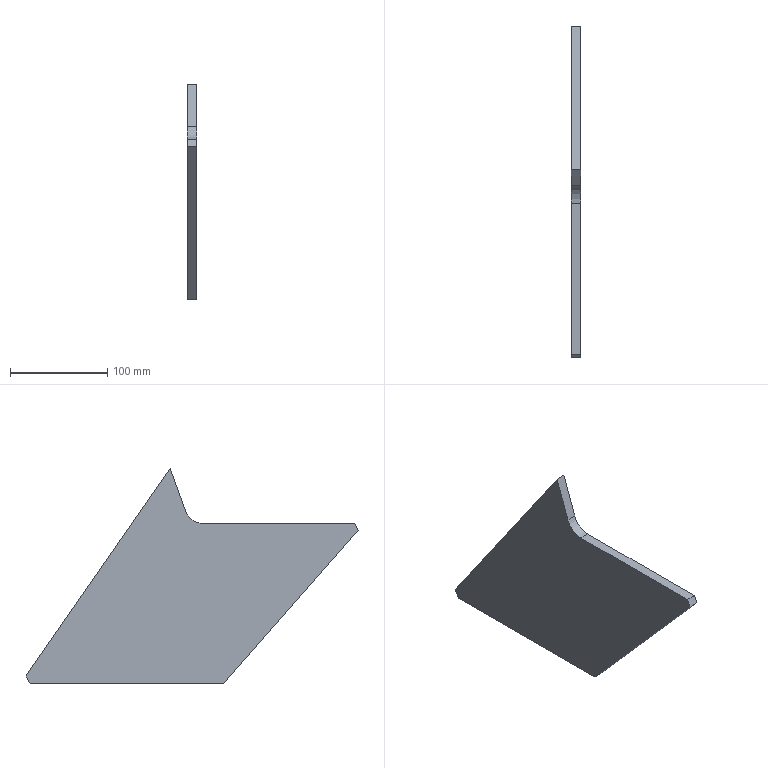Part | SolidWorks | features Extrusion 1 | 1 solid | 10 faces | box 10 x 341.699 x 222 mm | volume 386732 mm3 | plane 9 | cylinder 1 | commonest cylinder face diameters 40 x1
STEP:
#1=CARTESIAN_POINT('',(0.,6.601,157.488));
#2=VERTEX_POINT('',#1);
#3=CARTESIAN_POINT('',(0.,145.,0.));
#4=VERTEX_POINT('',#3);
#5=CARTESIAN_POINT('',(0.,6.601,157.488));
#6=DIRECTION('',(0.,0.6601,-0.7512));
#7=VECTOR('',#6,1000.);
#8=LINE('',#5,#7);
#9=EDGE_CURVE('',#2,#4,#8,.T.);
#10=ORIENTED_EDGE('',*,*,#9,.T.);
#11=CARTESIAN_POINT('',(10.,145.,0.));
#12=VERTEX_POINT('',#11);
#13=CARTESIAN_POINT('',(10.,145.,0.));
#14=DIRECTION('',(-1.,0.,0.));
#15=VECTOR('',#14,1000.);
#16=LINE('',#13,#15);
#17=EDGE_CURVE('',#12,#4,#16,.T.);
#18=ORIENTED_EDGE('',*,*,#17,.F.);
#19=CARTESIAN_POINT('',(10.,6.601,157.488));
#20=VERTEX_POINT('',#19);
#21=CARTESIAN_POINT('',(10.,6.601,157.488));
#22=DIRECTION('',(0.,0.6601,-0.7512));
#23=VECTOR('',#22,1000.);
#24=LINE('',#21,#23);
#25=EDGE_CURVE('',#20,#12,#24,.T.);
#26=ORIENTED_EDGE('',*,*,#25,.F.);
#27=CARTESIAN_POINT('',(10.,6.601,157.488));
#28=DIRECTION('',(-1.,0.,0.));
#29=VECTOR('',#28,1000.);
#30=LINE('',#27,#29);
#31=EDGE_CURVE('',#20,#2,#30,.T.);
#32=ORIENTED_EDGE('',*,*,#31,.T.);
#33=EDGE_LOOP('',(#10,#18,#26,#32));
#34=FACE_OUTER_BOUND('',#33,.T.);
#35=CARTESIAN_POINT('',(10.,6.601,157.488));
#36=DIRECTION('',(0.,0.7512,0.6601));
#37=DIRECTION('',(0.,-0.6601,0.7512));
#38=AXIS2_PLACEMENT_3D('',#35,#36,#37);
#39=PLANE('',#38);
#40=ADVANCED_FACE('',(#34),#39,.F.);
#41=CARTESIAN_POINT('',(0.,344.,0.));
#42=VERTEX_POINT('',#41);
#43=CARTESIAN_POINT('',(0.,145.,0.));
#44=DIRECTION('',(0.,1.,0.));
#45=VECTOR('',#44,1000.);
#46=LINE('',#43,#45);
#47=EDGE_CURVE('',#4,#42,#46,.T.);
#48=ORIENTED_EDGE('',*,*,#47,.T.);
#49=CARTESIAN_POINT('',(10.,344.,0.));
#50=VERTEX_POINT('',#49);
#51=CARTESIAN_POINT('',(10.,344.,0.));
#52=DIRECTION('',(-1.,0.,0.));
#53=VECTOR('',#52,1000.);
#54=LINE('',#51,#53);
#55=EDGE_CURVE('',#50,#42,#54,.T.);
#56=ORIENTED_EDGE('',*,*,#55,.F.);
#57=CARTESIAN_POINT('',(10.,145.,0.));
#58=DIRECTION('',(0.,1.,0.));
#59=VECTOR('',#58,1000.);
#60=LINE('',#57,#59);
#61=EDGE_CURVE('',#12,#50,#60,.T.);
#62=ORIENTED_EDGE('',*,*,#61,.F.);
#63=ORIENTED_EDGE('',*,*,#17,.T.);
#64=EDGE_LOOP('',(#48,#56,#62,#63));
#65=FACE_OUTER_BOUND('',#64,.T.);
#66=CARTESIAN_POINT('',(10.,145.,0.));
#67=DIRECTION('',(0.,0.,1.));
#68=DIRECTION('',(1.,0.,0.));
#69=AXIS2_PLACEMENT_3D('',#66,#67,#68);
#70=PLANE('',#69);
#71=ADVANCED_FACE('',(#65),#70,.F.);
#72=CARTESIAN_POINT('',(0.,348.3,8.217));
#73=VERTEX_POINT('',#72);
#74=CARTESIAN_POINT('',(0.,344.,0.));
#75=DIRECTION('',(0.,0.4637,0.886));
#76=VECTOR('',#75,1000.);
#77=LINE('',#74,#76);
#78=EDGE_CURVE('',#42,#73,#77,.T.);
#79=ORIENTED_EDGE('',*,*,#78,.T.);
#80=CARTESIAN_POINT('',(10.,348.3,8.217));
#81=VERTEX_POINT('',#80);
#82=CARTESIAN_POINT('',(10.,348.3,8.217));
#83=DIRECTION('',(-1.,0.,0.));
#84=VECTOR('',#83,1000.);
#85=LINE('',#82,#84);
#86=EDGE_CURVE('',#81,#73,#85,.T.);
#87=ORIENTED_EDGE('',*,*,#86,.F.);
#88=CARTESIAN_POINT('',(10.,344.,0.));
#89=DIRECTION('',(0.,0.4637,0.886));
#90=VECTOR('',#89,1000.);
#91=LINE('',#88,#90);
#92=EDGE_CURVE('',#50,#81,#91,.T.);
#93=ORIENTED_EDGE('',*,*,#92,.F.);
#94=ORIENTED_EDGE('',*,*,#55,.T.);
#95=EDGE_LOOP('',(#79,#87,#93,#94));
#96=FACE_OUTER_BOUND('',#95,.T.);
#97=CARTESIAN_POINT('',(10.,344.,0.));
#98=DIRECTION('',(0.,-0.886,0.4637));
#99=DIRECTION('',(0.,-0.4637,-0.886));
#100=AXIS2_PLACEMENT_3D('',#97,#98,#99);
#101=PLANE('',#100);
#102=ADVANCED_FACE('',(#96),#101,.F.);
#103=CARTESIAN_POINT('',(0.,200.,222.));
#104=VERTEX_POINT('',#103);
#105=CARTESIAN_POINT('',(0.,348.3,8.217));
#106=DIRECTION('',(0.,-0.57,0.8217));
#107=VECTOR('',#106,1000.);
#108=LINE('',#105,#107);
#109=EDGE_CURVE('',#73,#104,#108,.T.);
#110=ORIENTED_EDGE('',*,*,#109,.T.);
#111=CARTESIAN_POINT('',(10.,200.,222.));
#112=VERTEX_POINT('',#111);
#113=CARTESIAN_POINT('',(10.,200.,222.));
#114=DIRECTION('',(-1.,0.,0.));
#115=VECTOR('',#114,1000.);
#116=LINE('',#113,#115);
#117=EDGE_CURVE('',#112,#104,#116,.T.);
#118=ORIENTED_EDGE('',*,*,#117,.F.);
#119=CARTESIAN_POINT('',(10.,348.3,8.217));
#120=DIRECTION('',(0.,-0.57,0.8217));
#121=VECTOR('',#120,1000.);
#122=LINE('',#119,#121);
#123=EDGE_CURVE('',#81,#112,#122,.T.);
#124=ORIENTED_EDGE('',*,*,#123,.F.);
#125=ORIENTED_EDGE('',*,*,#86,.T.);
#126=EDGE_LOOP('',(#110,#118,#124,#125));
#127=FACE_OUTER_BOUND('',#126,.T.);
#128=CARTESIAN_POINT('',(10.,348.3,8.217));
#129=DIRECTION('',(0.,-0.8217,-0.57));
#130=DIRECTION('',(0.,0.57,-0.8217));
#131=AXIS2_PLACEMENT_3D('',#128,#129,#130);
#132=PLANE('',#131);
#133=ADVANCED_FACE('',(#127),#132,.F.);
#134=CARTESIAN_POINT('',(0.,184.259,178.231));
#135=VERTEX_POINT('',#134);
#136=CARTESIAN_POINT('',(0.,200.,222.));
#137=DIRECTION('',(0.,-0.3384,-0.941));
#138=VECTOR('',#137,1000.);
#139=LINE('',#136,#138);
#140=EDGE_CURVE('',#104,#135,#139,.T.);
#141=ORIENTED_EDGE('',*,*,#140,.T.);
#142=CARTESIAN_POINT('',(10.,184.259,178.231));
#143=VERTEX_POINT('',#142);
#144=CARTESIAN_POINT('',(10.,184.259,178.231));
#145=DIRECTION('',(-1.,0.,0.));
#146=VECTOR('',#145,1000.);
#147=LINE('',#144,#146);
#148=EDGE_CURVE('',#143,#135,#147,.T.);
#149=ORIENTED_EDGE('',*,*,#148,.F.);
#150=CARTESIAN_POINT('',(10.,200.,222.));
#151=DIRECTION('',(0.,-0.3384,-0.941));
#152=VECTOR('',#151,1000.);
#153=LINE('',#150,#152);
#154=EDGE_CURVE('',#112,#143,#153,.T.);
#155=ORIENTED_EDGE('',*,*,#154,.F.);
#156=ORIENTED_EDGE('',*,*,#117,.T.);
#157=EDGE_LOOP('',(#141,#149,#155,#156));
#158=FACE_OUTER_BOUND('',#157,.T.);
#159=CARTESIAN_POINT('',(10.,200.,222.));
#160=DIRECTION('',(0.,0.941,-0.3384));
#161=DIRECTION('',(0.,0.3384,0.941));
#162=AXIS2_PLACEMENT_3D('',#159,#160,#161);
#163=PLANE('',#162);
#164=ADVANCED_FACE('',(#158),#163,.F.);
#165=CARTESIAN_POINT('',(0.,165.439,165.));
#166=VERTEX_POINT('',#165);
#167=CARTESIAN_POINT('',(0.,165.439,185.));
#168=DIRECTION('',(-1.,0.,0.));
#169=DIRECTION('',(0.,0.,1.));
#170=AXIS2_PLACEMENT_3D('',#167,#168,#169);
#171=CIRCLE('',#170,20.);
#172=EDGE_CURVE('',#135,#166,#171,.T.);
#173=ORIENTED_EDGE('',*,*,#172,.T.);
#174=CARTESIAN_POINT('',(10.,165.439,165.));
#175=VERTEX_POINT('',#174);
#176=CARTESIAN_POINT('',(10.,165.439,165.));
#177=DIRECTION('',(-1.,0.,0.));
#178=VECTOR('',#177,1000.);
#179=LINE('',#176,#178);
#180=EDGE_CURVE('',#175,#166,#179,.T.);
#181=ORIENTED_EDGE('',*,*,#180,.F.);
#182=CARTESIAN_POINT('',(10.,165.439,185.));
#183=DIRECTION('',(-1.,0.,0.));
#184=DIRECTION('',(0.,0.,1.));
#185=AXIS2_PLACEMENT_3D('',#182,#183,#184);
#186=CIRCLE('',#185,20.);
#187=EDGE_CURVE('',#143,#175,#186,.T.);
#188=ORIENTED_EDGE('',*,*,#187,.F.);
#189=ORIENTED_EDGE('',*,*,#148,.T.);
#190=EDGE_LOOP('',(#173,#181,#188,#189));
#191=FACE_OUTER_BOUND('',#190,.T.);
#192=CARTESIAN_POINT('',(10.,165.439,185.));
#193=DIRECTION('',(-1.,0.,0.));
#194=DIRECTION('',(0.,0.,1.));
#195=AXIS2_PLACEMENT_3D('',#192,#193,#194);
#196=CYLINDRICAL_SURFACE('',#195,20.);
#197=ADVANCED_FACE('',(#191),#196,.F.);
#198=CARTESIAN_POINT('',(0.,10.,165.));
#199=VERTEX_POINT('',#198);
#200=CARTESIAN_POINT('',(0.,165.439,165.));
#201=DIRECTION('',(0.,-1.,0.));
#202=VECTOR('',#201,1000.);
#203=LINE('',#200,#202);
#204=EDGE_CURVE('',#166,#199,#203,.T.);
#205=ORIENTED_EDGE('',*,*,#204,.T.);
#206=CARTESIAN_POINT('',(10.,10.,165.));
#207=VERTEX_POINT('',#206);
#208=CARTESIAN_POINT('',(10.,10.,165.));
#209=DIRECTION('',(-1.,0.,0.));
#210=VECTOR('',#209,1000.);
#211=LINE('',#208,#210);
#212=EDGE_CURVE('',#207,#199,#211,.T.);
#213=ORIENTED_EDGE('',*,*,#212,.F.);
#214=CARTESIAN_POINT('',(10.,165.439,165.));
#215=DIRECTION('',(0.,-1.,0.));
#216=VECTOR('',#215,1000.);
#217=LINE('',#214,#216);
#218=EDGE_CURVE('',#175,#207,#217,.T.);
#219=ORIENTED_EDGE('',*,*,#218,.F.);
#220=ORIENTED_EDGE('',*,*,#180,.T.);
#221=EDGE_LOOP('',(#205,#213,#219,#220));
#222=FACE_OUTER_BOUND('',#221,.T.);
#223=CARTESIAN_POINT('',(10.,165.439,165.));
#224=DIRECTION('',(0.,0.,-1.));
#225=DIRECTION('',(0.,1.,0.));
#226=AXIS2_PLACEMENT_3D('',#223,#224,#225);
#227=PLANE('',#226);
#228=ADVANCED_FACE('',(#222),#227,.F.);
#229=CARTESIAN_POINT('',(0.,10.,165.));
#230=DIRECTION('',(0.,-0.4122,-0.9111));
#231=VECTOR('',#230,1000.);
#232=LINE('',#229,#231);
#233=EDGE_CURVE('',#199,#2,#232,.T.);
#234=ORIENTED_EDGE('',*,*,#233,.T.);
#235=ORIENTED_EDGE('',*,*,#31,.F.);
#236=CARTESIAN_POINT('',(10.,10.,165.));
#237=DIRECTION('',(0.,-0.4122,-0.9111));
#238=VECTOR('',#237,1000.);
#239=LINE('',#236,#238);
#240=EDGE_CURVE('',#207,#20,#239,.T.);
#241=ORIENTED_EDGE('',*,*,#240,.F.);
#242=ORIENTED_EDGE('',*,*,#212,.T.);
#243=EDGE_LOOP('',(#234,#235,#241,#242));
#244=FACE_OUTER_BOUND('',#243,.T.);
#245=CARTESIAN_POINT('',(10.,10.,165.));
#246=DIRECTION('',(0.,0.9111,-0.4122));
#247=DIRECTION('',(0.,0.4122,0.9111));
#248=AXIS2_PLACEMENT_3D('',#245,#246,#247);
#249=PLANE('',#248);
#250=ADVANCED_FACE('',(#244),#249,.F.);
#251=ORIENTED_EDGE('',*,*,#25,.T.);
#252=ORIENTED_EDGE('',*,*,#61,.T.);
#253=ORIENTED_EDGE('',*,*,#92,.T.);
#254=ORIENTED_EDGE('',*,*,#123,.T.);
#255=ORIENTED_EDGE('',*,*,#154,.T.);
#256=ORIENTED_EDGE('',*,*,#187,.T.);
#257=ORIENTED_EDGE('',*,*,#218,.T.);
#258=ORIENTED_EDGE('',*,*,#240,.T.);
#259=EDGE_LOOP('',(#251,#252,#253,#254,#255,#256,#257,#258));
#260=FACE_OUTER_BOUND('',#259,.T.);
#261=CARTESIAN_POINT('',(10.,165.439,185.));
#262=DIRECTION('',(-1.,0.,0.));
#263=DIRECTION('',(0.,0.,1.));
#264=AXIS2_PLACEMENT_3D('',#261,#262,#263);
#265=PLANE('',#264);
#266=ADVANCED_FACE('',(#260),#265,.F.);
#267=ORIENTED_EDGE('',*,*,#9,.F.);
#268=ORIENTED_EDGE('',*,*,#233,.F.);
#269=ORIENTED_EDGE('',*,*,#204,.F.);
#270=ORIENTED_EDGE('',*,*,#172,.F.);
#271=ORIENTED_EDGE('',*,*,#140,.F.);
#272=ORIENTED_EDGE('',*,*,#109,.F.);
#273=ORIENTED_EDGE('',*,*,#78,.F.);
#274=ORIENTED_EDGE('',*,*,#47,.F.);
#275=EDGE_LOOP('',(#267,#268,#269,#270,#271,#272,#273,#274));
#276=FACE_OUTER_BOUND('',#275,.T.);
#277=CARTESIAN_POINT('',(0.,165.439,185.));
#278=DIRECTION('',(-1.,0.,0.));
#279=DIRECTION('',(0.,0.,1.));
#280=AXIS2_PLACEMENT_3D('',#277,#278,#279);
#281=PLANE('',#280);
#282=ADVANCED_FACE('',(#276),#281,.T.);
#283=CLOSED_SHELL('',(#40,#71,#102,#133,#164,#197,#228,#250,#266,#282));
#284=MANIFOLD_SOLID_BREP('',#283);
#285=CARTESIAN_POINT('',(0.,0.,0.));
#286=DIRECTION('',(0.,0.,1.));
#287=DIRECTION('',(1.,0.,0.));
#288=AXIS2_PLACEMENT_3D('',#285,#286,#287);
#289=(LENGTH_UNIT()NAMED_UNIT(*)SI_UNIT(.MILLI.,.METRE.));
#290=UNCERTAINTY_MEASURE_WITH_UNIT(LENGTH_MEASURE(0.00001),#289,'','');
#291=(NAMED_UNIT(*)PLANE_ANGLE_UNIT()SI_UNIT($,.RADIAN.));
#292=(NAMED_UNIT(*)SI_UNIT($,.STERADIAN.)SOLID_ANGLE_UNIT());
#293=(GEOMETRIC_REPRESENTATION_CONTEXT(3)GLOBAL_UNCERTAINTY_ASSIGNED_CONTEXT((#290))GLOBAL_UNIT_ASSIGNED_CONTEXT((#289,#291,#292))REPRESENTATION_CONTEXT('',''));
#294=ADVANCED_BREP_SHAPE_REPRESENTATION('',(#284,#288),#293);